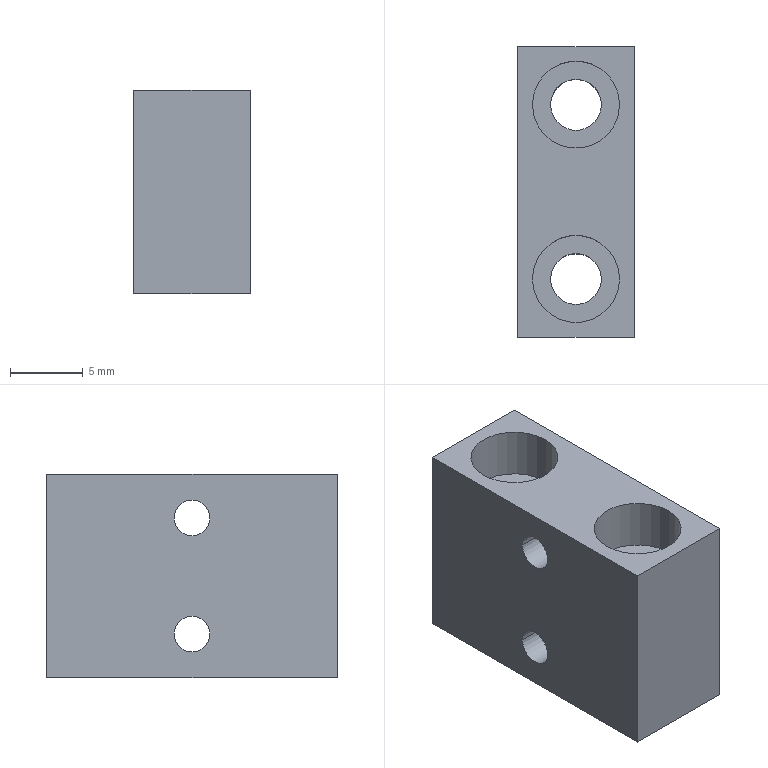Part | SolidWorks | features BaseBody 1 | 1 solid | 20 faces | box 8 x 20 x 14 mm | volume 1764 mm3 | cylinder 12 | plane 8 | commonest cylinder face diameters 2.459 x4 3.5 x4 6 x4
STEP:
#1=CARTESIAN_POINT('',(27.61,-4.583,11.));
#2=VERTEX_POINT('',#1);
#3=CARTESIAN_POINT('',(27.61,-2.124,11.));
#4=VERTEX_POINT('',#3);
#5=CARTESIAN_POINT('',(27.61,-3.354,11.));
#6=DIRECTION('',(1.,0.,0.));
#7=DIRECTION('',(0.,1.,0.));
#8=AXIS2_PLACEMENT_3D('',#5,#6,#7);
#9=CIRCLE('',#8,1.23);
#10=EDGE_CURVE('',#2,#4,#9,.T.);
#11=ORIENTED_EDGE('',*,*,#10,.F.);
#12=CARTESIAN_POINT('',(35.61,-4.583,11.));
#13=VERTEX_POINT('',#12);
#14=CARTESIAN_POINT('',(9.92,-4.583,11.));
#15=DIRECTION('',(1.,0.,0.));
#16=VECTOR('',#15,1000.);
#17=LINE('',#14,#16);
#18=EDGE_CURVE('',#2,#13,#17,.T.);
#19=ORIENTED_EDGE('',*,*,#18,.T.);
#20=CARTESIAN_POINT('',(35.61,-2.124,11.));
#21=VERTEX_POINT('',#20);
#22=CARTESIAN_POINT('',(35.61,-3.354,11.));
#23=DIRECTION('',(-1.,0.,0.));
#24=DIRECTION('',(0.,1.,0.));
#25=AXIS2_PLACEMENT_3D('',#22,#23,#24);
#26=CIRCLE('',#25,1.23);
#27=EDGE_CURVE('',#21,#13,#26,.T.);
#28=ORIENTED_EDGE('',*,*,#27,.F.);
#29=CARTESIAN_POINT('',(9.92,-2.124,11.));
#30=DIRECTION('',(1.,0.,0.));
#31=VECTOR('',#30,1000.);
#32=LINE('',#29,#31);
#33=EDGE_CURVE('',#4,#21,#32,.T.);
#34=ORIENTED_EDGE('',*,*,#33,.F.);
#35=EDGE_LOOP('',(#11,#19,#28,#34));
#36=FACE_OUTER_BOUND('',#35,.T.);
#37=CARTESIAN_POINT('',(9.92,-3.354,11.));
#38=DIRECTION('',(1.,0.,0.));
#39=DIRECTION('',(0.,1.,0.));
#40=AXIS2_PLACEMENT_3D('',#37,#38,#39);
#41=CYLINDRICAL_SURFACE('',#40,1.23);
#42=ADVANCED_FACE('',(#36),#41,.F.);
#43=CARTESIAN_POINT('',(27.61,-4.583,3.));
#44=VERTEX_POINT('',#43);
#45=CARTESIAN_POINT('',(27.61,-2.124,3.));
#46=VERTEX_POINT('',#45);
#47=CARTESIAN_POINT('',(27.61,-3.354,3.));
#48=DIRECTION('',(1.,0.,0.));
#49=DIRECTION('',(0.,1.,0.));
#50=AXIS2_PLACEMENT_3D('',#47,#48,#49);
#51=CIRCLE('',#50,1.23);
#52=EDGE_CURVE('',#44,#46,#51,.T.);
#53=ORIENTED_EDGE('',*,*,#52,.F.);
#54=CARTESIAN_POINT('',(35.61,-4.583,3.));
#55=VERTEX_POINT('',#54);
#56=CARTESIAN_POINT('',(9.92,-4.583,3.));
#57=DIRECTION('',(1.,0.,0.));
#58=VECTOR('',#57,1000.);
#59=LINE('',#56,#58);
#60=EDGE_CURVE('',#44,#55,#59,.T.);
#61=ORIENTED_EDGE('',*,*,#60,.T.);
#62=CARTESIAN_POINT('',(35.61,-2.124,3.));
#63=VERTEX_POINT('',#62);
#64=CARTESIAN_POINT('',(35.61,-3.354,3.));
#65=DIRECTION('',(-1.,0.,0.));
#66=DIRECTION('',(0.,1.,0.));
#67=AXIS2_PLACEMENT_3D('',#64,#65,#66);
#68=CIRCLE('',#67,1.23);
#69=EDGE_CURVE('',#63,#55,#68,.T.);
#70=ORIENTED_EDGE('',*,*,#69,.F.);
#71=CARTESIAN_POINT('',(9.92,-2.124,3.));
#72=DIRECTION('',(1.,0.,0.));
#73=VECTOR('',#72,1000.);
#74=LINE('',#71,#73);
#75=EDGE_CURVE('',#46,#63,#74,.T.);
#76=ORIENTED_EDGE('',*,*,#75,.F.);
#77=EDGE_LOOP('',(#53,#61,#70,#76));
#78=FACE_OUTER_BOUND('',#77,.T.);
#79=CARTESIAN_POINT('',(9.92,-3.354,3.));
#80=DIRECTION('',(1.,0.,0.));
#81=DIRECTION('',(0.,1.,0.));
#82=AXIS2_PLACEMENT_3D('',#79,#80,#81);
#83=CYLINDRICAL_SURFACE('',#82,1.23);
#84=ADVANCED_FACE('',(#78),#83,.F.);
#85=CARTESIAN_POINT('',(33.36,2.646,0.));
#86=VERTEX_POINT('',#85);
#87=CARTESIAN_POINT('',(29.86,2.646,0.));
#88=VERTEX_POINT('',#87);
#89=CARTESIAN_POINT('',(31.61,2.646,0.));
#90=DIRECTION('',(0.,0.,-1.));
#91=DIRECTION('',(1.,0.,0.));
#92=AXIS2_PLACEMENT_3D('',#89,#90,#91);
#93=CIRCLE('',#92,1.75);
#94=EDGE_CURVE('',#86,#88,#93,.T.);
#95=ORIENTED_EDGE('',*,*,#94,.T.);
#96=CARTESIAN_POINT('',(29.86,2.646,10.5));
#97=VERTEX_POINT('',#96);
#98=CARTESIAN_POINT('',(29.86,2.646,-11.69));
#99=DIRECTION('',(0.,0.,1.));
#100=VECTOR('',#99,1000.);
#101=LINE('',#98,#100);
#102=EDGE_CURVE('',#88,#97,#101,.T.);
#103=ORIENTED_EDGE('',*,*,#102,.T.);
#104=CARTESIAN_POINT('',(33.36,2.646,10.5));
#105=VERTEX_POINT('',#104);
#106=CARTESIAN_POINT('',(31.61,2.646,10.5));
#107=DIRECTION('',(0.,0.,-1.));
#108=DIRECTION('',(1.,0.,0.));
#109=AXIS2_PLACEMENT_3D('',#106,#107,#108);
#110=CIRCLE('',#109,1.75);
#111=EDGE_CURVE('',#105,#97,#110,.T.);
#112=ORIENTED_EDGE('',*,*,#111,.F.);
#113=CARTESIAN_POINT('',(33.36,2.646,-11.69));
#114=DIRECTION('',(0.,0.,1.));
#115=VECTOR('',#114,1000.);
#116=LINE('',#113,#115);
#117=EDGE_CURVE('',#86,#105,#116,.T.);
#118=ORIENTED_EDGE('',*,*,#117,.F.);
#119=EDGE_LOOP('',(#95,#103,#112,#118));
#120=FACE_OUTER_BOUND('',#119,.T.);
#121=CARTESIAN_POINT('',(31.61,2.646,-11.69));
#122=DIRECTION('',(0.,0.,1.));
#123=DIRECTION('',(1.,0.,0.));
#124=AXIS2_PLACEMENT_3D('',#121,#122,#123);
#125=CYLINDRICAL_SURFACE('',#124,1.75);
#126=ADVANCED_FACE('',(#120),#125,.F.);
#127=CARTESIAN_POINT('',(33.36,-9.354,0.));
#128=VERTEX_POINT('',#127);
#129=CARTESIAN_POINT('',(29.86,-9.354,0.));
#130=VERTEX_POINT('',#129);
#131=CARTESIAN_POINT('',(31.61,-9.354,0.));
#132=DIRECTION('',(0.,0.,-1.));
#133=DIRECTION('',(1.,0.,0.));
#134=AXIS2_PLACEMENT_3D('',#131,#132,#133);
#135=CIRCLE('',#134,1.75);
#136=EDGE_CURVE('',#128,#130,#135,.T.);
#137=ORIENTED_EDGE('',*,*,#136,.T.);
#138=CARTESIAN_POINT('',(29.86,-9.354,10.5));
#139=VERTEX_POINT('',#138);
#140=CARTESIAN_POINT('',(29.86,-9.354,-11.69));
#141=DIRECTION('',(0.,0.,1.));
#142=VECTOR('',#141,1000.);
#143=LINE('',#140,#142);
#144=EDGE_CURVE('',#130,#139,#143,.T.);
#145=ORIENTED_EDGE('',*,*,#144,.T.);
#146=CARTESIAN_POINT('',(33.36,-9.354,10.5));
#147=VERTEX_POINT('',#146);
#148=CARTESIAN_POINT('',(31.61,-9.354,10.5));
#149=DIRECTION('',(0.,0.,-1.));
#150=DIRECTION('',(1.,0.,0.));
#151=AXIS2_PLACEMENT_3D('',#148,#149,#150);
#152=CIRCLE('',#151,1.75);
#153=EDGE_CURVE('',#147,#139,#152,.T.);
#154=ORIENTED_EDGE('',*,*,#153,.F.);
#155=CARTESIAN_POINT('',(33.36,-9.354,-11.69));
#156=DIRECTION('',(0.,0.,1.));
#157=VECTOR('',#156,1000.);
#158=LINE('',#155,#157);
#159=EDGE_CURVE('',#128,#147,#158,.T.);
#160=ORIENTED_EDGE('',*,*,#159,.F.);
#161=EDGE_LOOP('',(#137,#145,#154,#160));
#162=FACE_OUTER_BOUND('',#161,.T.);
#163=CARTESIAN_POINT('',(31.61,-9.354,-11.69));
#164=DIRECTION('',(0.,0.,1.));
#165=DIRECTION('',(1.,0.,0.));
#166=AXIS2_PLACEMENT_3D('',#163,#164,#165);
#167=CYLINDRICAL_SURFACE('',#166,1.75);
#168=ADVANCED_FACE('',(#162),#167,.F.);
#169=CARTESIAN_POINT('',(28.61,2.646,10.5));
#170=VERTEX_POINT('',#169);
#171=CARTESIAN_POINT('',(34.61,2.646,10.5));
#172=VERTEX_POINT('',#171);
#173=CARTESIAN_POINT('',(31.61,2.646,10.5));
#174=DIRECTION('',(0.,0.,1.));
#175=DIRECTION('',(1.,0.,0.));
#176=AXIS2_PLACEMENT_3D('',#173,#174,#175);
#177=CIRCLE('',#176,3.);
#178=EDGE_CURVE('',#170,#172,#177,.T.);
#179=ORIENTED_EDGE('',*,*,#178,.F.);
#180=CARTESIAN_POINT('',(28.61,2.646,14.));
#181=VERTEX_POINT('',#180);
#182=CARTESIAN_POINT('',(28.61,2.646,12.25));
#183=DIRECTION('',(0.,0.,1.));
#184=VECTOR('',#183,1000.);
#185=LINE('',#182,#184);
#186=EDGE_CURVE('',#170,#181,#185,.T.);
#187=ORIENTED_EDGE('',*,*,#186,.T.);
#188=CARTESIAN_POINT('',(34.61,2.646,14.));
#189=VERTEX_POINT('',#188);
#190=CARTESIAN_POINT('',(31.61,2.646,14.));
#191=DIRECTION('',(0.,0.,-1.));
#192=DIRECTION('',(1.,0.,0.));
#193=AXIS2_PLACEMENT_3D('',#190,#191,#192);
#194=CIRCLE('',#193,3.);
#195=EDGE_CURVE('',#189,#181,#194,.T.);
#196=ORIENTED_EDGE('',*,*,#195,.F.);
#197=CARTESIAN_POINT('',(34.61,2.646,12.25));
#198=DIRECTION('',(0.,0.,1.));
#199=VECTOR('',#198,1000.);
#200=LINE('',#197,#199);
#201=EDGE_CURVE('',#172,#189,#200,.T.);
#202=ORIENTED_EDGE('',*,*,#201,.F.);
#203=EDGE_LOOP('',(#179,#187,#196,#202));
#204=FACE_OUTER_BOUND('',#203,.T.);
#205=CARTESIAN_POINT('',(31.61,2.646,12.25));
#206=DIRECTION('',(0.,0.,1.));
#207=DIRECTION('',(1.,0.,0.));
#208=AXIS2_PLACEMENT_3D('',#205,#206,#207);
#209=CYLINDRICAL_SURFACE('',#208,3.);
#210=ADVANCED_FACE('',(#204),#209,.F.);
#211=CARTESIAN_POINT('',(28.61,-9.354,10.5));
#212=VERTEX_POINT('',#211);
#213=CARTESIAN_POINT('',(34.61,-9.354,10.5));
#214=VERTEX_POINT('',#213);
#215=CARTESIAN_POINT('',(31.61,-9.354,10.5));
#216=DIRECTION('',(0.,0.,1.));
#217=DIRECTION('',(1.,0.,0.));
#218=AXIS2_PLACEMENT_3D('',#215,#216,#217);
#219=CIRCLE('',#218,3.);
#220=EDGE_CURVE('',#212,#214,#219,.T.);
#221=ORIENTED_EDGE('',*,*,#220,.F.);
#222=CARTESIAN_POINT('',(28.61,-9.354,14.));
#223=VERTEX_POINT('',#222);
#224=CARTESIAN_POINT('',(28.61,-9.354,12.25));
#225=DIRECTION('',(0.,0.,1.));
#226=VECTOR('',#225,1000.);
#227=LINE('',#224,#226);
#228=EDGE_CURVE('',#212,#223,#227,.T.);
#229=ORIENTED_EDGE('',*,*,#228,.T.);
#230=CARTESIAN_POINT('',(34.61,-9.354,14.));
#231=VERTEX_POINT('',#230);
#232=CARTESIAN_POINT('',(31.61,-9.354,14.));
#233=DIRECTION('',(0.,0.,-1.));
#234=DIRECTION('',(1.,0.,0.));
#235=AXIS2_PLACEMENT_3D('',#232,#233,#234);
#236=CIRCLE('',#235,3.);
#237=EDGE_CURVE('',#231,#223,#236,.T.);
#238=ORIENTED_EDGE('',*,*,#237,.F.);
#239=CARTESIAN_POINT('',(34.61,-9.354,12.25));
#240=DIRECTION('',(0.,0.,1.));
#241=VECTOR('',#240,1000.);
#242=LINE('',#239,#241);
#243=EDGE_CURVE('',#214,#231,#242,.T.);
#244=ORIENTED_EDGE('',*,*,#243,.F.);
#245=EDGE_LOOP('',(#221,#229,#238,#244));
#246=FACE_OUTER_BOUND('',#245,.T.);
#247=CARTESIAN_POINT('',(31.61,-9.354,12.25));
#248=DIRECTION('',(0.,0.,1.));
#249=DIRECTION('',(1.,0.,0.));
#250=AXIS2_PLACEMENT_3D('',#247,#248,#249);
#251=CYLINDRICAL_SURFACE('',#250,3.);
#252=ADVANCED_FACE('',(#246),#251,.F.);
#253=ORIENTED_EDGE('',*,*,#27,.T.);
#254=CARTESIAN_POINT('',(35.61,-3.354,11.));
#255=DIRECTION('',(-1.,0.,0.));
#256=DIRECTION('',(0.,1.,0.));
#257=AXIS2_PLACEMENT_3D('',#254,#255,#256);
#258=CIRCLE('',#257,1.23);
#259=EDGE_CURVE('',#13,#21,#258,.T.);
#260=ORIENTED_EDGE('',*,*,#259,.T.);
#261=EDGE_LOOP('',(#253,#260));
#262=FACE_BOUND('',#261,.T.);
#263=ORIENTED_EDGE('',*,*,#69,.T.);
#264=CARTESIAN_POINT('',(35.61,-3.354,3.));
#265=DIRECTION('',(-1.,0.,0.));
#266=DIRECTION('',(0.,1.,0.));
#267=AXIS2_PLACEMENT_3D('',#264,#265,#266);
#268=CIRCLE('',#267,1.23);
#269=EDGE_CURVE('',#55,#63,#268,.T.);
#270=ORIENTED_EDGE('',*,*,#269,.T.);
#271=EDGE_LOOP('',(#263,#270));
#272=FACE_BOUND('',#271,.T.);
#273=CARTESIAN_POINT('',(35.61,-13.354,0.));
#274=VERTEX_POINT('',#273);
#275=CARTESIAN_POINT('',(35.61,6.646,0.));
#276=VERTEX_POINT('',#275);
#277=CARTESIAN_POINT('',(35.61,6.646,0.));
#278=DIRECTION('',(0.,1.,0.));
#279=VECTOR('',#278,1000.);
#280=LINE('',#277,#279);
#281=EDGE_CURVE('',#274,#276,#280,.T.);
#282=ORIENTED_EDGE('',*,*,#281,.T.);
#283=CARTESIAN_POINT('',(35.61,6.646,14.));
#284=VERTEX_POINT('',#283);
#285=CARTESIAN_POINT('',(35.61,6.646,0.));
#286=DIRECTION('',(0.,0.,1.));
#287=VECTOR('',#286,1000.);
#288=LINE('',#285,#287);
#289=EDGE_CURVE('',#276,#284,#288,.T.);
#290=ORIENTED_EDGE('',*,*,#289,.T.);
#291=CARTESIAN_POINT('',(35.61,-13.354,14.));
#292=VERTEX_POINT('',#291);
#293=CARTESIAN_POINT('',(35.61,6.646,14.));
#294=DIRECTION('',(0.,-1.,0.));
#295=VECTOR('',#294,1000.);
#296=LINE('',#293,#295);
#297=EDGE_CURVE('',#284,#292,#296,.T.);
#298=ORIENTED_EDGE('',*,*,#297,.T.);
#299=CARTESIAN_POINT('',(35.61,-13.354,0.));
#300=DIRECTION('',(0.,0.,-1.));
#301=VECTOR('',#300,1000.);
#302=LINE('',#299,#301);
#303=EDGE_CURVE('',#292,#274,#302,.T.);
#304=ORIENTED_EDGE('',*,*,#303,.T.);
#305=EDGE_LOOP('',(#282,#290,#298,#304));
#306=FACE_OUTER_BOUND('',#305,.T.);
#307=CARTESIAN_POINT('',(35.61,6.646,0.));
#308=DIRECTION('',(1.,0.,0.));
#309=DIRECTION('',(0.,0.,-1.));
#310=AXIS2_PLACEMENT_3D('',#307,#308,#309);
#311=PLANE('',#310);
#312=ADVANCED_FACE('',(#262,#272,#306),#311,.T.);
#313=ORIENTED_EDGE('',*,*,#18,.F.);
#314=CARTESIAN_POINT('',(27.61,-3.354,11.));
#315=DIRECTION('',(1.,0.,0.));
#316=DIRECTION('',(0.,1.,0.));
#317=AXIS2_PLACEMENT_3D('',#314,#315,#316);
#318=CIRCLE('',#317,1.23);
#319=EDGE_CURVE('',#4,#2,#318,.T.);
#320=ORIENTED_EDGE('',*,*,#319,.F.);
#321=ORIENTED_EDGE('',*,*,#33,.T.);
#322=ORIENTED_EDGE('',*,*,#259,.F.);
#323=EDGE_LOOP('',(#313,#320,#321,#322));
#324=FACE_OUTER_BOUND('',#323,.T.);
#325=CARTESIAN_POINT('',(9.92,-3.354,11.));
#326=DIRECTION('',(1.,0.,0.));
#327=DIRECTION('',(0.,1.,0.));
#328=AXIS2_PLACEMENT_3D('',#325,#326,#327);
#329=CYLINDRICAL_SURFACE('',#328,1.23);
#330=ADVANCED_FACE('',(#324),#329,.F.);
#331=ORIENTED_EDGE('',*,*,#60,.F.);
#332=CARTESIAN_POINT('',(27.61,-3.354,3.));
#333=DIRECTION('',(1.,0.,0.));
#334=DIRECTION('',(0.,1.,0.));
#335=AXIS2_PLACEMENT_3D('',#332,#333,#334);
#336=CIRCLE('',#335,1.23);
#337=EDGE_CURVE('',#46,#44,#336,.T.);
#338=ORIENTED_EDGE('',*,*,#337,.F.);
#339=ORIENTED_EDGE('',*,*,#75,.T.);
#340=ORIENTED_EDGE('',*,*,#269,.F.);
#341=EDGE_LOOP('',(#331,#338,#339,#340));
#342=FACE_OUTER_BOUND('',#341,.T.);
#343=CARTESIAN_POINT('',(9.92,-3.354,3.));
#344=DIRECTION('',(1.,0.,0.));
#345=DIRECTION('',(0.,1.,0.));
#346=AXIS2_PLACEMENT_3D('',#343,#344,#345);
#347=CYLINDRICAL_SURFACE('',#346,1.23);
#348=ADVANCED_FACE('',(#342),#347,.F.);
#349=CARTESIAN_POINT('',(27.61,6.646,0.));
#350=VERTEX_POINT('',#349);
#351=CARTESIAN_POINT('',(27.61,6.646,0.));
#352=DIRECTION('',(-1.,0.,0.));
#353=VECTOR('',#352,1000.);
#354=LINE('',#351,#353);
#355=EDGE_CURVE('',#276,#350,#354,.T.);
#356=ORIENTED_EDGE('',*,*,#355,.T.);
#357=CARTESIAN_POINT('',(27.61,6.646,14.));
#358=VERTEX_POINT('',#357);
#359=CARTESIAN_POINT('',(27.61,6.646,0.));
#360=DIRECTION('',(0.,0.,1.));
#361=VECTOR('',#360,1000.);
#362=LINE('',#359,#361);
#363=EDGE_CURVE('',#350,#358,#362,.T.);
#364=ORIENTED_EDGE('',*,*,#363,.T.);
#365=CARTESIAN_POINT('',(27.61,6.646,14.));
#366=DIRECTION('',(1.,0.,0.));
#367=VECTOR('',#366,1000.);
#368=LINE('',#365,#367);
#369=EDGE_CURVE('',#358,#284,#368,.T.);
#370=ORIENTED_EDGE('',*,*,#369,.T.);
#371=ORIENTED_EDGE('',*,*,#289,.F.);
#372=EDGE_LOOP('',(#356,#364,#370,#371));
#373=FACE_OUTER_BOUND('',#372,.T.);
#374=CARTESIAN_POINT('',(27.61,6.646,0.));
#375=DIRECTION('',(0.,1.,0.));
#376=DIRECTION('',(0.,0.,1.));
#377=AXIS2_PLACEMENT_3D('',#374,#375,#376);
#378=PLANE('',#377);
#379=ADVANCED_FACE('',(#373),#378,.T.);
#380=ORIENTED_EDGE('',*,*,#94,.F.);
#381=CARTESIAN_POINT('',(31.61,2.646,0.));
#382=DIRECTION('',(0.,0.,-1.));
#383=DIRECTION('',(1.,0.,0.));
#384=AXIS2_PLACEMENT_3D('',#381,#382,#383);
#385=CIRCLE('',#384,1.75);
#386=EDGE_CURVE('',#88,#86,#385,.T.);
#387=ORIENTED_EDGE('',*,*,#386,.F.);
#388=EDGE_LOOP('',(#380,#387));
#389=FACE_BOUND('',#388,.T.);
#390=ORIENTED_EDGE('',*,*,#136,.F.);
#391=CARTESIAN_POINT('',(31.61,-9.354,0.));
#392=DIRECTION('',(0.,0.,-1.));
#393=DIRECTION('',(1.,0.,0.));
#394=AXIS2_PLACEMENT_3D('',#391,#392,#393);
#395=CIRCLE('',#394,1.75);
#396=EDGE_CURVE('',#130,#128,#395,.T.);
#397=ORIENTED_EDGE('',*,*,#396,.F.);
#398=EDGE_LOOP('',(#390,#397));
#399=FACE_BOUND('',#398,.T.);
#400=ORIENTED_EDGE('',*,*,#281,.F.);
#401=CARTESIAN_POINT('',(27.61,-13.354,0.));
#402=VERTEX_POINT('',#401);
#403=CARTESIAN_POINT('',(31.61,-13.354,0.));
#404=DIRECTION('',(1.,0.,0.));
#405=VECTOR('',#404,1000.);
#406=LINE('',#403,#405);
#407=EDGE_CURVE('',#402,#274,#406,.T.);
#408=ORIENTED_EDGE('',*,*,#407,.F.);
#409=CARTESIAN_POINT('',(27.61,-3.354,0.));
#410=DIRECTION('',(0.,-1.,0.));
#411=VECTOR('',#410,1000.);
#412=LINE('',#409,#411);
#413=EDGE_CURVE('',#350,#402,#412,.T.);
#414=ORIENTED_EDGE('',*,*,#413,.F.);
#415=ORIENTED_EDGE('',*,*,#355,.F.);
#416=EDGE_LOOP('',(#400,#408,#414,#415));
#417=FACE_OUTER_BOUND('',#416,.T.);
#418=CARTESIAN_POINT('',(31.61,-3.354,0.));
#419=DIRECTION('',(0.,0.,1.));
#420=DIRECTION('',(1.,0.,0.));
#421=AXIS2_PLACEMENT_3D('',#418,#419,#420);
#422=PLANE('',#421);
#423=ADVANCED_FACE('',(#389,#399,#417),#422,.F.);
#424=ORIENTED_EDGE('',*,*,#407,.T.);
#425=ORIENTED_EDGE('',*,*,#303,.F.);
#426=CARTESIAN_POINT('',(27.61,-13.354,14.));
#427=VERTEX_POINT('',#426);
#428=CARTESIAN_POINT('',(35.61,-13.354,14.));
#429=DIRECTION('',(-1.,0.,0.));
#430=VECTOR('',#429,1000.);
#431=LINE('',#428,#430);
#432=EDGE_CURVE('',#292,#427,#431,.T.);
#433=ORIENTED_EDGE('',*,*,#432,.T.);
#434=CARTESIAN_POINT('',(27.61,-13.354,0.));
#435=DIRECTION('',(0.,0.,-1.));
#436=VECTOR('',#435,1000.);
#437=LINE('',#434,#436);
#438=EDGE_CURVE('',#427,#402,#437,.T.);
#439=ORIENTED_EDGE('',*,*,#438,.T.);
#440=EDGE_LOOP('',(#424,#425,#433,#439));
#441=FACE_OUTER_BOUND('',#440,.T.);
#442=CARTESIAN_POINT('',(35.61,-13.354,0.));
#443=DIRECTION('',(0.,-1.,0.));
#444=DIRECTION('',(0.,0.,-1.));
#445=AXIS2_PLACEMENT_3D('',#442,#443,#444);
#446=PLANE('',#445);
#447=ADVANCED_FACE('',(#441),#446,.T.);
#448=ORIENTED_EDGE('',*,*,#195,.T.);
#449=CARTESIAN_POINT('',(31.61,2.646,14.));
#450=DIRECTION('',(0.,0.,-1.));
#451=DIRECTION('',(1.,0.,0.));
#452=AXIS2_PLACEMENT_3D('',#449,#450,#451);
#453=CIRCLE('',#452,3.);
#454=EDGE_CURVE('',#181,#189,#453,.T.);
#455=ORIENTED_EDGE('',*,*,#454,.T.);
#456=EDGE_LOOP('',(#448,#455));
#457=FACE_BOUND('',#456,.T.);
#458=ORIENTED_EDGE('',*,*,#237,.T.);
#459=CARTESIAN_POINT('',(31.61,-9.354,14.));
#460=DIRECTION('',(0.,0.,-1.));
#461=DIRECTION('',(1.,0.,0.));
#462=AXIS2_PLACEMENT_3D('',#459,#460,#461);
#463=CIRCLE('',#462,3.);
#464=EDGE_CURVE('',#223,#231,#463,.T.);
#465=ORIENTED_EDGE('',*,*,#464,.T.);
#466=EDGE_LOOP('',(#458,#465));
#467=FACE_BOUND('',#466,.T.);
#468=CARTESIAN_POINT('',(27.61,-3.354,14.));
#469=DIRECTION('',(0.,-1.,0.));
#470=VECTOR('',#469,1000.);
#471=LINE('',#468,#470);
#472=EDGE_CURVE('',#358,#427,#471,.T.);
#473=ORIENTED_EDGE('',*,*,#472,.T.);
#474=ORIENTED_EDGE('',*,*,#432,.F.);
#475=ORIENTED_EDGE('',*,*,#297,.F.);
#476=ORIENTED_EDGE('',*,*,#369,.F.);
#477=EDGE_LOOP('',(#473,#474,#475,#476));
#478=FACE_OUTER_BOUND('',#477,.T.);
#479=CARTESIAN_POINT('',(31.61,-3.354,14.));
#480=DIRECTION('',(0.,0.,1.));
#481=DIRECTION('',(1.,0.,0.));
#482=AXIS2_PLACEMENT_3D('',#479,#480,#481);
#483=PLANE('',#482);
#484=ADVANCED_FACE('',(#457,#467,#478),#483,.T.);
#485=ORIENTED_EDGE('',*,*,#319,.T.);
#486=ORIENTED_EDGE('',*,*,#10,.T.);
#487=EDGE_LOOP('',(#485,#486));
#488=FACE_BOUND('',#487,.T.);
#489=ORIENTED_EDGE('',*,*,#337,.T.);
#490=ORIENTED_EDGE('',*,*,#52,.T.);
#491=EDGE_LOOP('',(#489,#490));
#492=FACE_BOUND('',#491,.T.);
#493=ORIENTED_EDGE('',*,*,#413,.T.);
#494=ORIENTED_EDGE('',*,*,#438,.F.);
#495=ORIENTED_EDGE('',*,*,#472,.F.);
#496=ORIENTED_EDGE('',*,*,#363,.F.);
#497=EDGE_LOOP('',(#493,#494,#495,#496));
#498=FACE_OUTER_BOUND('',#497,.T.);
#499=CARTESIAN_POINT('',(27.61,-13.354,0.));
#500=DIRECTION('',(-1.,0.,0.));
#501=DIRECTION('',(0.,0.,1.));
#502=AXIS2_PLACEMENT_3D('',#499,#500,#501);
#503=PLANE('',#502);
#504=ADVANCED_FACE('',(#488,#492,#498),#503,.T.);
#505=ORIENTED_EDGE('',*,*,#102,.F.);
#506=ORIENTED_EDGE('',*,*,#386,.T.);
#507=ORIENTED_EDGE('',*,*,#117,.T.);
#508=CARTESIAN_POINT('',(31.61,2.646,10.5));
#509=DIRECTION('',(0.,0.,-1.));
#510=DIRECTION('',(1.,0.,0.));
#511=AXIS2_PLACEMENT_3D('',#508,#509,#510);
#512=CIRCLE('',#511,1.75);
#513=EDGE_CURVE('',#97,#105,#512,.T.);
#514=ORIENTED_EDGE('',*,*,#513,.F.);
#515=EDGE_LOOP('',(#505,#506,#507,#514));
#516=FACE_OUTER_BOUND('',#515,.T.);
#517=CARTESIAN_POINT('',(31.61,2.646,-11.69));
#518=DIRECTION('',(0.,0.,1.));
#519=DIRECTION('',(1.,0.,0.));
#520=AXIS2_PLACEMENT_3D('',#517,#518,#519);
#521=CYLINDRICAL_SURFACE('',#520,1.75);
#522=ADVANCED_FACE('',(#516),#521,.F.);
#523=ORIENTED_EDGE('',*,*,#144,.F.);
#524=ORIENTED_EDGE('',*,*,#396,.T.);
#525=ORIENTED_EDGE('',*,*,#159,.T.);
#526=CARTESIAN_POINT('',(31.61,-9.354,10.5));
#527=DIRECTION('',(0.,0.,-1.));
#528=DIRECTION('',(1.,0.,0.));
#529=AXIS2_PLACEMENT_3D('',#526,#527,#528);
#530=CIRCLE('',#529,1.75);
#531=EDGE_CURVE('',#139,#147,#530,.T.);
#532=ORIENTED_EDGE('',*,*,#531,.F.);
#533=EDGE_LOOP('',(#523,#524,#525,#532));
#534=FACE_OUTER_BOUND('',#533,.T.);
#535=CARTESIAN_POINT('',(31.61,-9.354,-11.69));
#536=DIRECTION('',(0.,0.,1.));
#537=DIRECTION('',(1.,0.,0.));
#538=AXIS2_PLACEMENT_3D('',#535,#536,#537);
#539=CYLINDRICAL_SURFACE('',#538,1.75);
#540=ADVANCED_FACE('',(#534),#539,.F.);
#541=ORIENTED_EDGE('',*,*,#186,.F.);
#542=CARTESIAN_POINT('',(31.61,2.646,10.5));
#543=DIRECTION('',(0.,0.,1.));
#544=DIRECTION('',(1.,0.,0.));
#545=AXIS2_PLACEMENT_3D('',#542,#543,#544);
#546=CIRCLE('',#545,3.);
#547=EDGE_CURVE('',#172,#170,#546,.T.);
#548=ORIENTED_EDGE('',*,*,#547,.F.);
#549=ORIENTED_EDGE('',*,*,#201,.T.);
#550=ORIENTED_EDGE('',*,*,#454,.F.);
#551=EDGE_LOOP('',(#541,#548,#549,#550));
#552=FACE_OUTER_BOUND('',#551,.T.);
#553=CARTESIAN_POINT('',(31.61,2.646,12.25));
#554=DIRECTION('',(0.,0.,1.));
#555=DIRECTION('',(1.,0.,0.));
#556=AXIS2_PLACEMENT_3D('',#553,#554,#555);
#557=CYLINDRICAL_SURFACE('',#556,3.);
#558=ADVANCED_FACE('',(#552),#557,.F.);
#559=ORIENTED_EDGE('',*,*,#228,.F.);
#560=CARTESIAN_POINT('',(31.61,-9.354,10.5));
#561=DIRECTION('',(0.,0.,1.));
#562=DIRECTION('',(1.,0.,0.));
#563=AXIS2_PLACEMENT_3D('',#560,#561,#562);
#564=CIRCLE('',#563,3.);
#565=EDGE_CURVE('',#214,#212,#564,.T.);
#566=ORIENTED_EDGE('',*,*,#565,.F.);
#567=ORIENTED_EDGE('',*,*,#243,.T.);
#568=ORIENTED_EDGE('',*,*,#464,.F.);
#569=EDGE_LOOP('',(#559,#566,#567,#568));
#570=FACE_OUTER_BOUND('',#569,.T.);
#571=CARTESIAN_POINT('',(31.61,-9.354,12.25));
#572=DIRECTION('',(0.,0.,1.));
#573=DIRECTION('',(1.,0.,0.));
#574=AXIS2_PLACEMENT_3D('',#571,#572,#573);
#575=CYLINDRICAL_SURFACE('',#574,3.);
#576=ADVANCED_FACE('',(#570),#575,.F.);
#577=ORIENTED_EDGE('',*,*,#111,.T.);
#578=ORIENTED_EDGE('',*,*,#513,.T.);
#579=EDGE_LOOP('',(#577,#578));
#580=FACE_BOUND('',#579,.T.);
#581=ORIENTED_EDGE('',*,*,#547,.T.);
#582=ORIENTED_EDGE('',*,*,#178,.T.);
#583=EDGE_LOOP('',(#581,#582));
#584=FACE_OUTER_BOUND('',#583,.T.);
#585=CARTESIAN_POINT('',(31.61,2.646,10.5));
#586=DIRECTION('',(0.,0.,1.));
#587=DIRECTION('',(1.,0.,0.));
#588=AXIS2_PLACEMENT_3D('',#585,#586,#587);
#589=PLANE('',#588);
#590=ADVANCED_FACE('',(#580,#584),#589,.T.);
#591=ORIENTED_EDGE('',*,*,#153,.T.);
#592=ORIENTED_EDGE('',*,*,#531,.T.);
#593=EDGE_LOOP('',(#591,#592));
#594=FACE_BOUND('',#593,.T.);
#595=ORIENTED_EDGE('',*,*,#565,.T.);
#596=ORIENTED_EDGE('',*,*,#220,.T.);
#597=EDGE_LOOP('',(#595,#596));
#598=FACE_OUTER_BOUND('',#597,.T.);
#599=CARTESIAN_POINT('',(31.61,-9.354,10.5));
#600=DIRECTION('',(0.,0.,1.));
#601=DIRECTION('',(1.,0.,0.));
#602=AXIS2_PLACEMENT_3D('',#599,#600,#601);
#603=PLANE('',#602);
#604=ADVANCED_FACE('',(#594,#598),#603,.T.);
#605=CLOSED_SHELL('',(#42,#84,#126,#168,#210,#252,#312,#330,#348,#379,#423,#447,#484,#504,#522,#540,#558,#576,#590,#604));
#606=MANIFOLD_SOLID_BREP('',#605);
#607=CARTESIAN_POINT('',(0.,0.,0.));
#608=DIRECTION('',(0.,0.,1.));
#609=DIRECTION('',(1.,0.,0.));
#610=AXIS2_PLACEMENT_3D('',#607,#608,#609);
#611=(LENGTH_UNIT()NAMED_UNIT(*)SI_UNIT(.MILLI.,.METRE.));
#612=UNCERTAINTY_MEASURE_WITH_UNIT(LENGTH_MEASURE(0.00001),#611,'','');
#613=(NAMED_UNIT(*)PLANE_ANGLE_UNIT()SI_UNIT($,.RADIAN.));
#614=(NAMED_UNIT(*)SI_UNIT($,.STERADIAN.)SOLID_ANGLE_UNIT());
#615=(GEOMETRIC_REPRESENTATION_CONTEXT(3)GLOBAL_UNCERTAINTY_ASSIGNED_CONTEXT((#612))GLOBAL_UNIT_ASSIGNED_CONTEXT((#611,#613,#614))REPRESENTATION_CONTEXT('',''));
#616=ADVANCED_BREP_SHAPE_REPRESENTATION('',(#606,#610),#615);